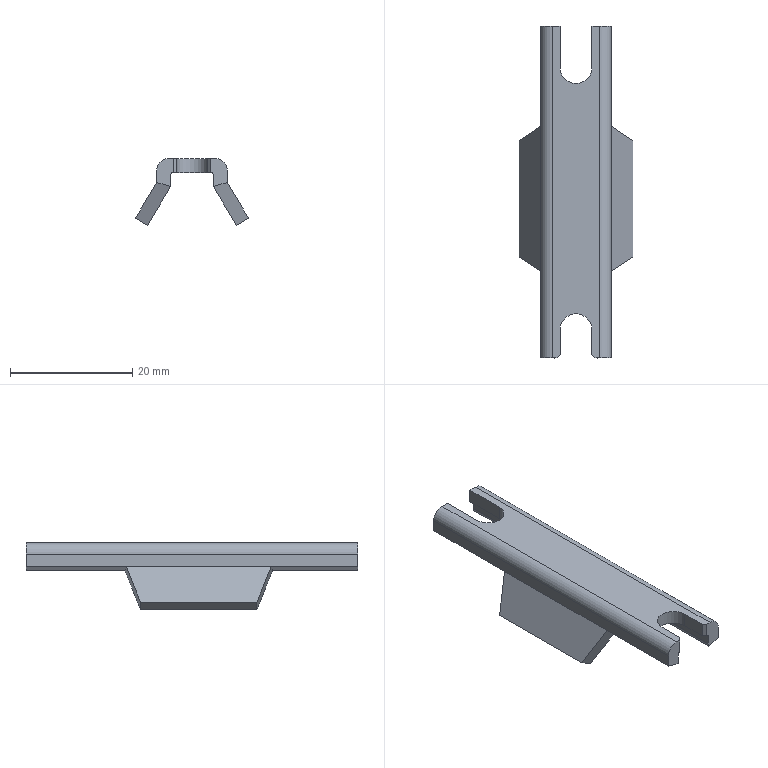Part | STEP file | AC40-04-KSTV-38JNR_AC3009A Spacer Front Plate | 1 solid | 38 faces | box 18.505 x 54.2 x 10.913 mm | volume 2347 mm3 | plane 30 | cylinder 8 | commonest cylinder face diameters 0.6 x2 3.2 x2 3.8 x2 5.2 x2